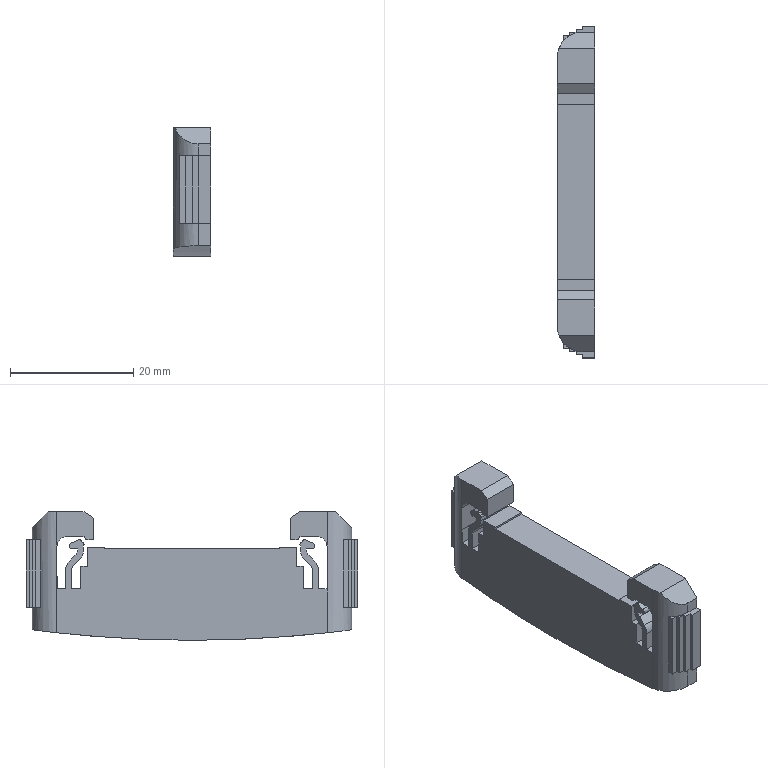Part | STEP file | [OP-26751]-Part-1 | 1 solid | 99 faces | box 6 x 53.8 x 20.8 mm | volume 4707 mm3 | plane 77 | cylinder 22 | commonest cylinder face diameters 0.6 x6 2 x4 4 x4 1 x2 3.4 x2 8 x2